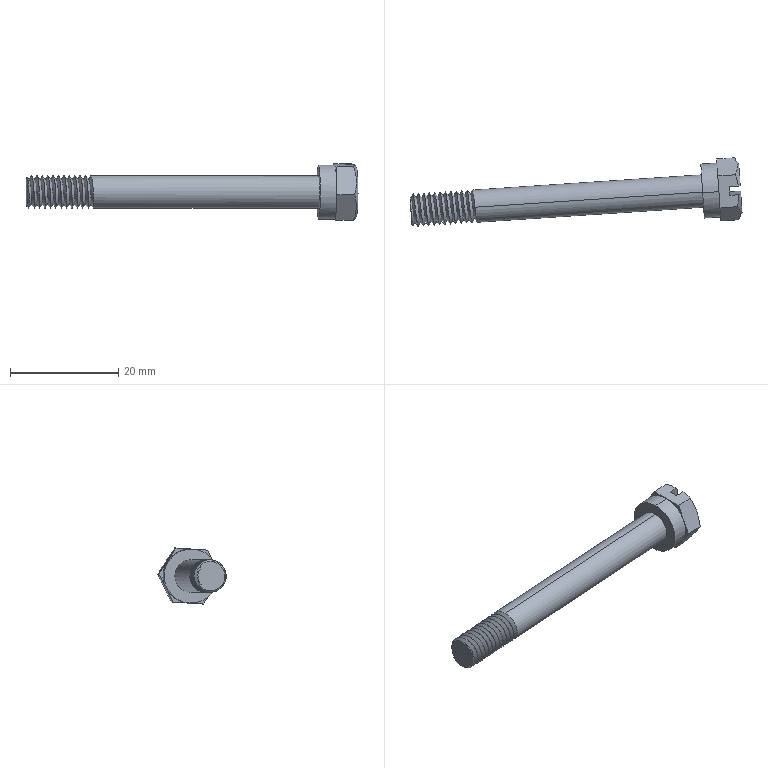Part | SolidWorks | features BaseBody 1 | 1 solid | 56 faces | box 61.328 x 12.638 x 10.359 mm | volume 2000 mm3 | cylinder 27 | plane 22 | cone 5 | spline 2 | commonest cylinder face diameters 6 x25 10 x2